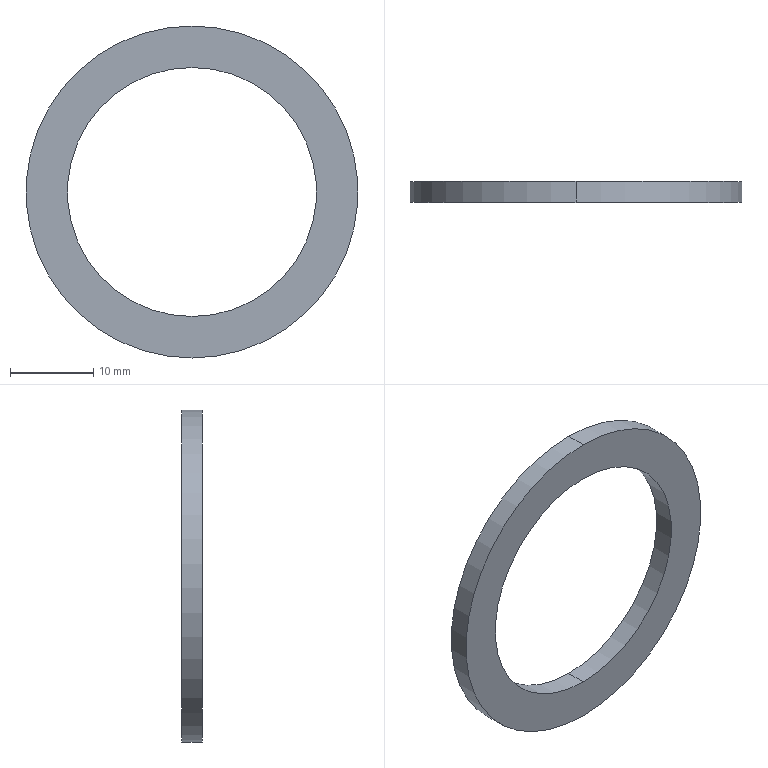Part | SolidWorks | features MBimport 1 | 1 solid | 6 faces | box 40 x 2.5 x 40 mm | volume 1374 mm3 | cylinder 4 | plane 2 | commonest cylinder face diameters 30 x2 40 x2
STEP:
#1=CARTESIAN_POINT('',(0.,32.016,-15.));
#2=VERTEX_POINT('',#1);
#3=CARTESIAN_POINT('',(0.,32.016,15.));
#4=VERTEX_POINT('',#3);
#5=CARTESIAN_POINT('',(0.,32.016,0.));
#6=DIRECTION('',(0.,-1.,0.));
#7=DIRECTION('',(0.,0.,-1.));
#8=AXIS2_PLACEMENT_3D('',#5,#6,#7);
#9=CIRCLE('',#8,15.);
#10=EDGE_CURVE('',#2,#4,#9,.T.);
#11=ORIENTED_EDGE('',*,*,#10,.T.);
#12=CARTESIAN_POINT('',(0.,32.016,0.));
#13=DIRECTION('',(0.,-1.,0.));
#14=DIRECTION('',(0.,0.,-1.));
#15=AXIS2_PLACEMENT_3D('',#12,#13,#14);
#16=CIRCLE('',#15,15.);
#17=EDGE_CURVE('',#4,#2,#16,.T.);
#18=ORIENTED_EDGE('',*,*,#17,.T.);
#19=EDGE_LOOP('',(#11,#18));
#20=FACE_BOUND('',#19,.T.);
#21=CARTESIAN_POINT('',(0.,32.016,-20.));
#22=VERTEX_POINT('',#21);
#23=CARTESIAN_POINT('',(0.,32.016,20.));
#24=VERTEX_POINT('',#23);
#25=CARTESIAN_POINT('',(0.,32.016,0.));
#26=DIRECTION('',(0.,-1.,0.));
#27=DIRECTION('',(0.,0.,-1.));
#28=AXIS2_PLACEMENT_3D('',#25,#26,#27);
#29=CIRCLE('',#28,20.);
#30=EDGE_CURVE('',#22,#24,#29,.T.);
#31=ORIENTED_EDGE('',*,*,#30,.F.);
#32=CARTESIAN_POINT('',(0.,32.016,0.));
#33=DIRECTION('',(0.,-1.,0.));
#34=DIRECTION('',(0.,0.,-1.));
#35=AXIS2_PLACEMENT_3D('',#32,#33,#34);
#36=CIRCLE('',#35,20.);
#37=EDGE_CURVE('',#24,#22,#36,.T.);
#38=ORIENTED_EDGE('',*,*,#37,.F.);
#39=EDGE_LOOP('',(#31,#38));
#40=FACE_OUTER_BOUND('',#39,.T.);
#41=CARTESIAN_POINT('',(-20.,32.016,0.));
#42=DIRECTION('',(0.,-1.,0.));
#43=DIRECTION('',(0.,0.,-1.));
#44=AXIS2_PLACEMENT_3D('',#41,#42,#43);
#45=PLANE('',#44);
#46=ADVANCED_FACE('',(#20,#40),#45,.F.);
#47=CARTESIAN_POINT('',(0.,29.516,15.));
#48=VERTEX_POINT('',#47);
#49=CARTESIAN_POINT('',(0.,0.,15.));
#50=DIRECTION('',(0.,-1.,0.));
#51=VECTOR('',#50,1000.);
#52=LINE('',#49,#51);
#53=EDGE_CURVE('',#4,#48,#52,.T.);
#54=ORIENTED_EDGE('',*,*,#53,.F.);
#55=ORIENTED_EDGE('',*,*,#10,.F.);
#56=CARTESIAN_POINT('',(0.,29.516,-15.));
#57=VERTEX_POINT('',#56);
#58=CARTESIAN_POINT('',(0.,0.,-15.));
#59=DIRECTION('',(0.,-1.,0.));
#60=VECTOR('',#59,1000.);
#61=LINE('',#58,#60);
#62=EDGE_CURVE('',#2,#57,#61,.T.);
#63=ORIENTED_EDGE('',*,*,#62,.T.);
#64=CARTESIAN_POINT('',(0.,29.516,0.));
#65=DIRECTION('',(0.,-1.,0.));
#66=DIRECTION('',(0.,0.,-1.));
#67=AXIS2_PLACEMENT_3D('',#64,#65,#66);
#68=CIRCLE('',#67,15.);
#69=EDGE_CURVE('',#57,#48,#68,.T.);
#70=ORIENTED_EDGE('',*,*,#69,.T.);
#71=EDGE_LOOP('',(#54,#55,#63,#70));
#72=FACE_OUTER_BOUND('',#71,.T.);
#73=CARTESIAN_POINT('',(0.,0.,0.));
#74=DIRECTION('',(0.,-1.,0.));
#75=DIRECTION('',(0.,0.,-1.));
#76=AXIS2_PLACEMENT_3D('',#73,#74,#75);
#77=CYLINDRICAL_SURFACE('',#76,15.);
#78=ADVANCED_FACE('',(#72),#77,.F.);
#79=ORIENTED_EDGE('',*,*,#69,.F.);
#80=CARTESIAN_POINT('',(0.,29.516,0.));
#81=DIRECTION('',(0.,-1.,0.));
#82=DIRECTION('',(0.,0.,-1.));
#83=AXIS2_PLACEMENT_3D('',#80,#81,#82);
#84=CIRCLE('',#83,15.);
#85=EDGE_CURVE('',#48,#57,#84,.T.);
#86=ORIENTED_EDGE('',*,*,#85,.F.);
#87=EDGE_LOOP('',(#79,#86));
#88=FACE_BOUND('',#87,.T.);
#89=CARTESIAN_POINT('',(0.,29.516,-20.));
#90=VERTEX_POINT('',#89);
#91=CARTESIAN_POINT('',(0.,29.516,20.));
#92=VERTEX_POINT('',#91);
#93=CARTESIAN_POINT('',(0.,29.516,0.));
#94=DIRECTION('',(0.,-1.,0.));
#95=DIRECTION('',(0.,0.,-1.));
#96=AXIS2_PLACEMENT_3D('',#93,#94,#95);
#97=CIRCLE('',#96,20.);
#98=EDGE_CURVE('',#90,#92,#97,.T.);
#99=ORIENTED_EDGE('',*,*,#98,.T.);
#100=CARTESIAN_POINT('',(0.,29.516,0.));
#101=DIRECTION('',(0.,-1.,0.));
#102=DIRECTION('',(0.,0.,-1.));
#103=AXIS2_PLACEMENT_3D('',#100,#101,#102);
#104=CIRCLE('',#103,20.);
#105=EDGE_CURVE('',#92,#90,#104,.T.);
#106=ORIENTED_EDGE('',*,*,#105,.T.);
#107=EDGE_LOOP('',(#99,#106));
#108=FACE_OUTER_BOUND('',#107,.T.);
#109=CARTESIAN_POINT('',(-20.,29.516,0.));
#110=DIRECTION('',(0.,1.,0.));
#111=DIRECTION('',(1.,0.,0.));
#112=AXIS2_PLACEMENT_3D('',#109,#110,#111);
#113=PLANE('',#112);
#114=ADVANCED_FACE('',(#88,#108),#113,.F.);
#115=CARTESIAN_POINT('',(0.,0.,20.));
#116=DIRECTION('',(0.,-1.,0.));
#117=VECTOR('',#116,1000.);
#118=LINE('',#115,#117);
#119=EDGE_CURVE('',#24,#92,#118,.T.);
#120=ORIENTED_EDGE('',*,*,#119,.F.);
#121=ORIENTED_EDGE('',*,*,#37,.T.);
#122=CARTESIAN_POINT('',(0.,0.,-20.));
#123=DIRECTION('',(0.,-1.,0.));
#124=VECTOR('',#123,1000.);
#125=LINE('',#122,#124);
#126=EDGE_CURVE('',#22,#90,#125,.T.);
#127=ORIENTED_EDGE('',*,*,#126,.T.);
#128=ORIENTED_EDGE('',*,*,#105,.F.);
#129=EDGE_LOOP('',(#120,#121,#127,#128));
#130=FACE_OUTER_BOUND('',#129,.T.);
#131=CARTESIAN_POINT('',(0.,0.,0.));
#132=DIRECTION('',(0.,-1.,0.));
#133=DIRECTION('',(0.,0.,-1.));
#134=AXIS2_PLACEMENT_3D('',#131,#132,#133);
#135=CYLINDRICAL_SURFACE('',#134,20.);
#136=ADVANCED_FACE('',(#130),#135,.T.);
#137=ORIENTED_EDGE('',*,*,#30,.T.);
#138=ORIENTED_EDGE('',*,*,#119,.T.);
#139=ORIENTED_EDGE('',*,*,#98,.F.);
#140=ORIENTED_EDGE('',*,*,#126,.F.);
#141=EDGE_LOOP('',(#137,#138,#139,#140));
#142=FACE_OUTER_BOUND('',#141,.T.);
#143=CARTESIAN_POINT('',(0.,0.,0.));
#144=DIRECTION('',(0.,-1.,0.));
#145=DIRECTION('',(0.,0.,-1.));
#146=AXIS2_PLACEMENT_3D('',#143,#144,#145);
#147=CYLINDRICAL_SURFACE('',#146,20.);
#148=ADVANCED_FACE('',(#142),#147,.T.);
#149=ORIENTED_EDGE('',*,*,#17,.F.);
#150=ORIENTED_EDGE('',*,*,#53,.T.);
#151=ORIENTED_EDGE('',*,*,#85,.T.);
#152=ORIENTED_EDGE('',*,*,#62,.F.);
#153=EDGE_LOOP('',(#149,#150,#151,#152));
#154=FACE_OUTER_BOUND('',#153,.T.);
#155=CARTESIAN_POINT('',(0.,0.,0.));
#156=DIRECTION('',(0.,-1.,0.));
#157=DIRECTION('',(0.,0.,-1.));
#158=AXIS2_PLACEMENT_3D('',#155,#156,#157);
#159=CYLINDRICAL_SURFACE('',#158,15.);
#160=ADVANCED_FACE('',(#154),#159,.F.);
#161=CLOSED_SHELL('',(#46,#78,#114,#136,#148,#160));
#162=MANIFOLD_SOLID_BREP('',#161);
#163=CARTESIAN_POINT('',(0.,0.,0.));
#164=DIRECTION('',(0.,0.,1.));
#165=DIRECTION('',(1.,0.,0.));
#166=AXIS2_PLACEMENT_3D('',#163,#164,#165);
#167=(LENGTH_UNIT()NAMED_UNIT(*)SI_UNIT(.MILLI.,.METRE.));
#168=UNCERTAINTY_MEASURE_WITH_UNIT(LENGTH_MEASURE(0.00001),#167,'','');
#169=(NAMED_UNIT(*)PLANE_ANGLE_UNIT()SI_UNIT($,.RADIAN.));
#170=(NAMED_UNIT(*)SI_UNIT($,.STERADIAN.)SOLID_ANGLE_UNIT());
#171=(GEOMETRIC_REPRESENTATION_CONTEXT(3)GLOBAL_UNCERTAINTY_ASSIGNED_CONTEXT((#168))GLOBAL_UNIT_ASSIGNED_CONTEXT((#167,#169,#170))REPRESENTATION_CONTEXT('',''));
#172=ADVANCED_BREP_SHAPE_REPRESENTATION('',(#162,#166),#171);